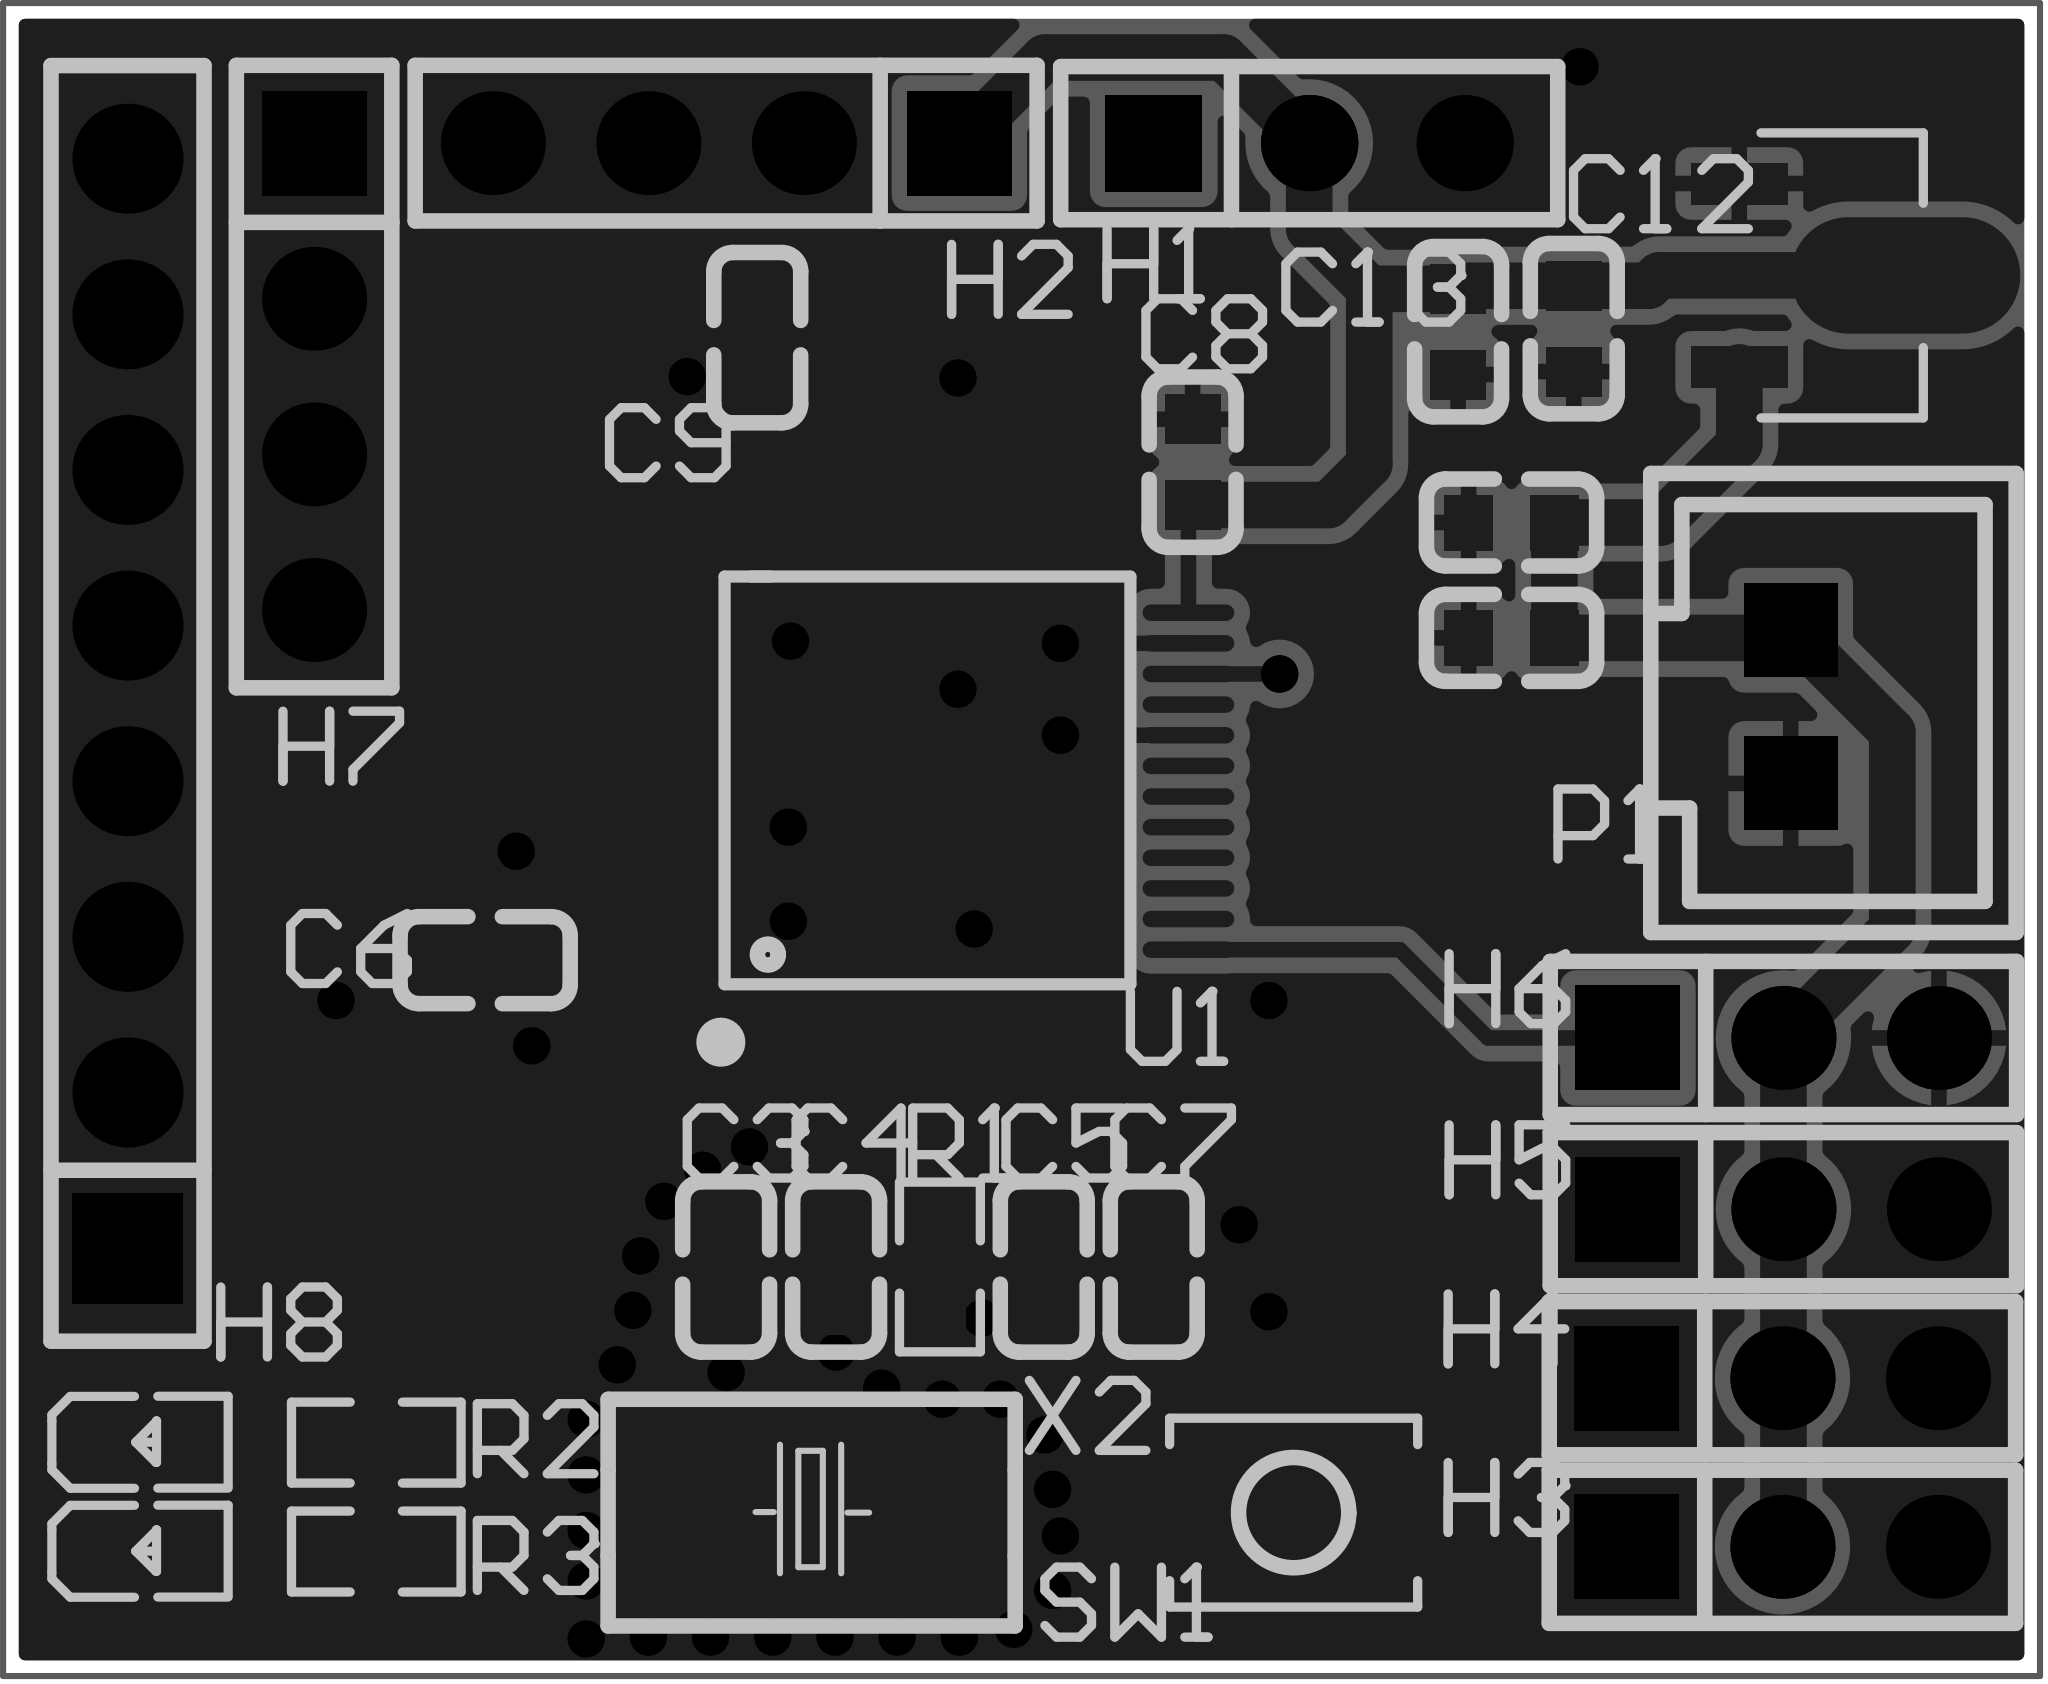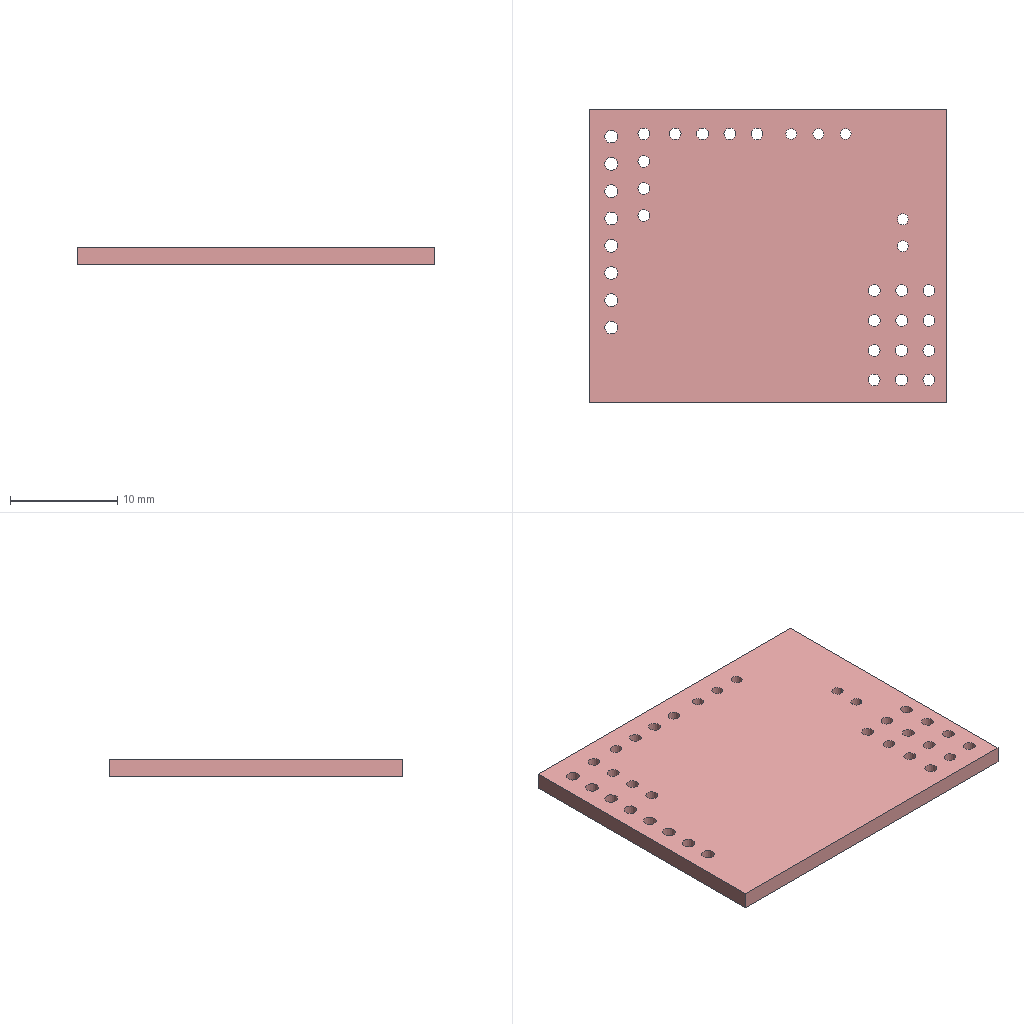Circuit board layout | Altium Designer | box 33.3 x 27.3 x 1.6 mm
Layer stack:
# Altium Designer layer stack of  (unit mm; dielectric type: 0 none, 1 core, 2 prepreg, 3 surface material)
index,name,kind,layer,copper_thickness_mm,dielectric_type,dielectric_thickness_mm,dielectric_material,dielectric_constant
0,Top Paste Mask Layer,other,,,,,,
1,Top Silkscreen Layer,other,,,,,,
2,Top Solder Mask Layer,dielectric,,,3,0.01,,3.3
3,Top Layer,copper,Top Layer,0.035,,,,
4,Dielectric1,dielectric,,,3,1.51,FR4,4.5
5,Bottom Layer,copper,Bottom Layer,0.035,,,,
6,Bottom Solder Mask Layer,dielectric,,,3,0.01,,3.3
7,Bottom Silkscreen Layer,other,,,,,,
8,Bottom Paste Mask Layer,other,,,,,,
# drill layer pairs: low layer,high layer
drill_pair,Top Layer,Bottom Layer
Part placement:
Designator,Comment,Layer,Footprint,Center-X(mm),Center-Y(mm),Rotation
C3,20pF,TopLayer,C0603,88.646,84.146,90
C4,20pF,TopLayer,C0603,90.442,84.146,90
C5,100nF,TopLayer,C0603,93.835,84.146,90
C6,100nF,TopLayer,C0603,84.709,89.154,0
C7,100nF,TopLayer,C0603,95.631,84.146,90
C8,100nF,TopLayer,C0603,96.266,97.282,270
C9,100nF,TopLayer,C0603,89.154,99.314,270
H2,PZ254V-11-04P,TopLayer,HDR-TH_4P-P2.54-V-M,88.646,102.489,180
R1,10kΩ,TopLayer,R0603,92.138,84.146,270
R2,680Ω,TopLayer,R0603,82.931,81.28,0
R3,680Ω,TopLayer,R0603,82.931,79.502,0
SW1,TS-1088-AR02016,TopLayer,SW-SMD_L3.9-W3.0-P4.45,97.917,80.137,0
U1,STM32F103C8T6,TopLayer,LQFP-48_L7.0-W7.0-P0.50-LS9.0-BL,91.948,92.075,0
X2,8MHz,TopLayer,CRYSTAL-SMD_L5.0-W3.2,90.043,80.137,180
H7,PZ254V-11-04P,TopLayer,HDR-TH_4P-P2.54-V-M,81.915,98.679,270
LED3,LTST-C190YKT,TopLayer,LED0603-RD,79.121,81.28,0
LED4,GL0603UB01,TopLayer,LED0603-RD_BLUE,79.121,79.502,0
C10,100nF,TopLayer,C0603,101.476,96.297,0
C11,10uF,TopLayer,C0603,101.476,94.414,0
C12,100nF,TopLayer,C0603,102.493,99.461,90
C13,10uF,TopLayer,C0603,100.603,99.411,90
H1,,TopLayer,HDR-TH_3P-P2.54-V-F,98.171,102.489,0
H3,,TopLayer,HDR-TH_3P-P2.54-V-M,105.902,79.579,0
H4,,TopLayer,HDR-TH_3P-P2.54-V-M,105.902,82.331,0
H5,,TopLayer,HDR-TH_3P-P2.54-V-M,105.918,85.09,0
H6,,TopLayer,HDR-TH_3P-P2.54-V-M,105.918,87.884,0
H8,,TopLayer,HDR-TH_8P-P2.54-V-F-1,78.867,93.345,90
P1,XH2.54直插座-2P,TopLayer,CONN-TH_XH2.54-2P,106.037,93.288,270
U2,AMS1117-1.2OFB,TopLayer,SOT-89-3_L4.5-W2.4-P1.50-LS4.0-BR,106.358,100.33,180
Pad and via stacks:
# Altium Designer via and pad stacks of  (unit mm). Each distinct definition once, with the count of objects using it.
# via: kind,start_layer,end_layer,hole_mm,diameter_mm,mode(0 simple;1 top-mid-bottom;2 full stack),diameter_per_layer,count,example_net
# pad: kind,layer,hole_mm,hole_type(0 round;1 square;2 slot),plating,top_size,top_shape(1 round;2 rect;3 octagon;9 rounded rect),mid_size,bottom_size,mode,footprint,size_per_layer,count,example
pad,Top Layer,0,0,plated,0.8x0.9,2,0.8x0.9,0.8x0.9,0,C0603,,22,C3.2
pad,Top Layer,0,0,plated,0.8065x0.864,2,0.8065x0.864,0.8065x0.864,0,R0603,,6,R1.2
pad,Top Layer,0,0,plated,1.23x1.86,2,1.23x1.86,1.23x1.86,0,SW-SMD_L3.9-W3.0-P4.45,,2,SW1.1
pad,Top Layer,0,0,plated,0.27x1.5,1,0.27x1.5,0.27x1.5,0,LQFP-48_L7.0-W7.0-P0.50-LS9.0-BL,,24,U1.1
pad,Top Layer,0,0,plated,1.5x0.27,1,1.5x0.27,1.5x0.27,0,LQFP-48_L7.0-W7.0-P0.50-LS9.0-BL,,24,U1.13
pad,Top Layer,0,0,plated,1.9x2.4,2,1.9x2.4,1.9x2.4,0,CRYSTAL-SMD_L5.0-W3.2,,2,X2.2
pad,Top Layer,0,0,plated,0.8x0.8,2,0.8x0.8,0.8x0.8,0,LED0603-RD,,2,LED3.2
pad,Top Layer,0,0,plated,0.8x0.8,2,0.8x0.8,0.8x0.8,0,LED0603-RD_BLUE,,2,LED4.1
pad,Top Layer,0,0,plated,0.95x0.95,1,0.95x0.95,0.95x0.95,0,SOT-89-3_L4.5-W2.4-P1.50-LS4.0-BR,,1,U2.2
pad,Top Layer,0,0,plated,1.575x0.672,2,1.575x0.672,1.575x0.672,0,SOT-89-3_L4.5-W2.4-P1.50-LS4.0-BR,,2,U2.3
pad,Multi-Layer,1.1,0,plated,1.7x1.7,2,1.7x1.7,1.7x1.7,0,HDR-TH_4P-P2.54-V-M,,2,H2.1
pad,Multi-Layer,1.1,0,plated,1.7x1.7,1,1.7x1.7,1.7x1.7,0,HDR-TH_4P-P2.54-V-M,,6,H2.2
pad,Multi-Layer,1.02,0,plated,1.575x1.575,1,1.575x1.575,1.575x1.575,0,HDR-TH_3P-P2.54-V-F,,2,H1.3
pad,Multi-Layer,1.02,0,plated,1.575x1.575,2,1.575x1.575,1.575x1.575,0,HDR-TH_3P-P2.54-V-F,,1,H1.1
pad,Multi-Layer,1.1,0,plated,1.7x1.7,2,1.7x1.7,1.7x1.7,0,HDR-TH_3P-P2.54-V-M,,4,H3.1
pad,Multi-Layer,1.1,0,plated,1.7x1.7,1,1.7x1.7,1.7x1.7,0,HDR-TH_3P-P2.54-V-M,,8,H3.2
pad,Multi-Layer,1.2,0,plated,1.8x1.8,2,1.8x1.8,1.8x1.8,0,HDR-TH_8P-P2.54-V-F-1,,1,H8.1
pad,Multi-Layer,1.2,0,plated,1.8x1.8,1,1.8x1.8,1.8x1.8,0,HDR-TH_8P-P2.54-V-F-1,,7,H8.2
pad,Multi-Layer,1,2,plated,1.524x1.524,2,1.524x1.524,1.524x1.524,0,CONN-TH_XH2.54-2P,,2,P1.1
via,Top Layer,Bottom Layer,0.3048,0.61,0,,45,PB8
Copper pours:
name,layer,net,type(0 solid;1 hatched;2 none)
Top Layer-GND,Top Layer,GND,0
Bottom Layer-GND,Bottom Layer,GND,0
Design rules, without the lines most boards share:
# Altium Designer design rules of  (exported by Altium Designer, unit mm)
# columns: name | kind | enabled | priority | scope1 | scope2 | descriptor | typed fields (field=value)
copperThickness1oz_2 | 2 | enabled | 2 | All | All | Width Constraint (Min=5mil) (Max=100mil) (Preferred=20mil) (All) |